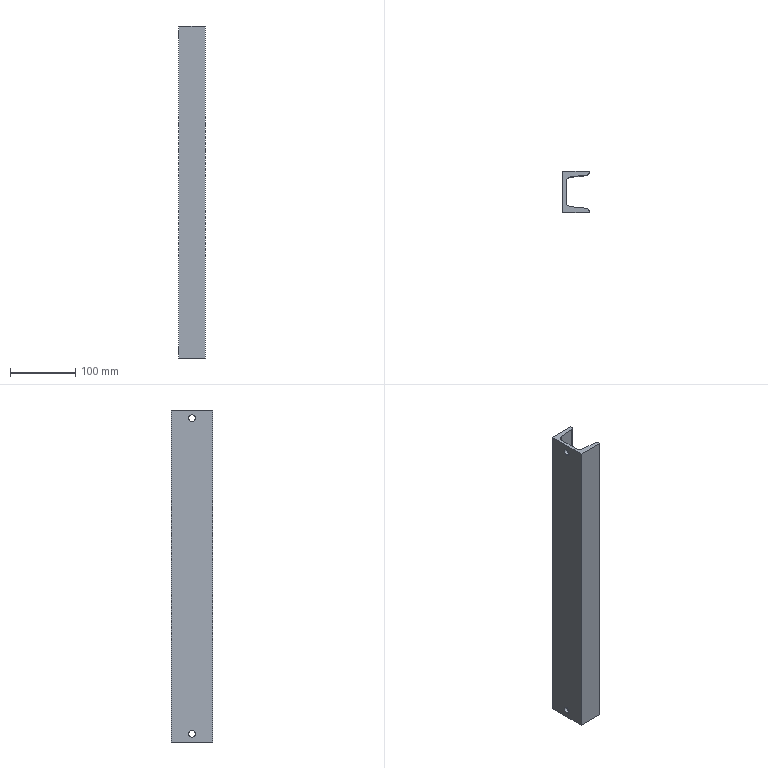Part | STEP file | 750038228 | 1 solid | 18 faces | box 40 x 63 x 510 mm | volume 429975 mm3 | plane 10 | cylinder 8 | commonest cylinder face diameters 10 x4 7.6 x2 15 x2
STEP:
#1=CARTESIAN_POINT('',(4.8,31.5,237.5));
#2=VERTEX_POINT('',#1);
#3=CARTESIAN_POINT('',(4.8,31.5,247.5));
#4=VERTEX_POINT('',#3);
#5=CARTESIAN_POINT('',(4.8,31.5,242.5));
#6=DIRECTION('',(-1.,0.,0.));
#7=DIRECTION('',(0.,0.,1.));
#8=AXIS2_PLACEMENT_3D('',#5,#6,#7);
#9=CIRCLE('',#8,5.);
#10=EDGE_CURVE('',#2,#4,#9,.T.);
#11=ORIENTED_EDGE('',*,*,#10,.F.);
#12=CARTESIAN_POINT('',(0.,31.5,237.5));
#13=VERTEX_POINT('',#12);
#14=CARTESIAN_POINT('',(55000.,31.5,237.5));
#15=DIRECTION('',(-1.,0.,0.));
#16=VECTOR('',#15,1000.);
#17=LINE('',#14,#16);
#18=EDGE_CURVE('',#2,#13,#17,.T.);
#19=ORIENTED_EDGE('',*,*,#18,.T.);
#20=CARTESIAN_POINT('',(0.,31.5,247.5));
#21=VERTEX_POINT('',#20);
#22=CARTESIAN_POINT('',(0.,31.5,242.5));
#23=DIRECTION('',(-1.,0.,0.));
#24=DIRECTION('',(0.,0.,1.));
#25=AXIS2_PLACEMENT_3D('',#22,#23,#24);
#26=CIRCLE('',#25,5.);
#27=EDGE_CURVE('',#13,#21,#26,.T.);
#28=ORIENTED_EDGE('',*,*,#27,.T.);
#29=CARTESIAN_POINT('',(55000.,31.5,247.5));
#30=DIRECTION('',(-1.,0.,0.));
#31=VECTOR('',#30,1000.);
#32=LINE('',#29,#31);
#33=EDGE_CURVE('',#4,#21,#32,.T.);
#34=ORIENTED_EDGE('',*,*,#33,.F.);
#35=EDGE_LOOP('',(#11,#19,#28,#34));
#36=FACE_OUTER_BOUND('',#35,.T.);
#37=CARTESIAN_POINT('',(55000.,31.5,242.5));
#38=DIRECTION('',(-1.,0.,0.));
#39=DIRECTION('',(0.,0.,1.));
#40=AXIS2_PLACEMENT_3D('',#37,#38,#39);
#41=CYLINDRICAL_SURFACE('',#40,5.);
#42=ADVANCED_FACE('',(#36),#41,.F.);
#43=CARTESIAN_POINT('',(4.8,31.5,-247.5));
#44=VERTEX_POINT('',#43);
#45=CARTESIAN_POINT('',(4.8,31.5,-237.5));
#46=VERTEX_POINT('',#45);
#47=CARTESIAN_POINT('',(4.8,31.5,-242.5));
#48=DIRECTION('',(-1.,0.,0.));
#49=DIRECTION('',(0.,0.,1.));
#50=AXIS2_PLACEMENT_3D('',#47,#48,#49);
#51=CIRCLE('',#50,5.);
#52=EDGE_CURVE('',#44,#46,#51,.T.);
#53=ORIENTED_EDGE('',*,*,#52,.F.);
#54=CARTESIAN_POINT('',(0.,31.5,-247.5));
#55=VERTEX_POINT('',#54);
#56=CARTESIAN_POINT('',(55000.,31.5,-247.5));
#57=DIRECTION('',(-1.,0.,0.));
#58=VECTOR('',#57,1000.);
#59=LINE('',#56,#58);
#60=EDGE_CURVE('',#44,#55,#59,.T.);
#61=ORIENTED_EDGE('',*,*,#60,.T.);
#62=CARTESIAN_POINT('',(0.,31.5,-237.5));
#63=VERTEX_POINT('',#62);
#64=CARTESIAN_POINT('',(0.,31.5,-242.5));
#65=DIRECTION('',(-1.,0.,0.));
#66=DIRECTION('',(0.,0.,1.));
#67=AXIS2_PLACEMENT_3D('',#64,#65,#66);
#68=CIRCLE('',#67,5.);
#69=EDGE_CURVE('',#55,#63,#68,.T.);
#70=ORIENTED_EDGE('',*,*,#69,.T.);
#71=CARTESIAN_POINT('',(55000.,31.5,-237.5));
#72=DIRECTION('',(-1.,0.,0.));
#73=VECTOR('',#72,1000.);
#74=LINE('',#71,#73);
#75=EDGE_CURVE('',#46,#63,#74,.T.);
#76=ORIENTED_EDGE('',*,*,#75,.F.);
#77=EDGE_LOOP('',(#53,#61,#70,#76));
#78=FACE_OUTER_BOUND('',#77,.T.);
#79=CARTESIAN_POINT('',(55000.,31.5,-242.5));
#80=DIRECTION('',(-1.,0.,0.));
#81=DIRECTION('',(0.,0.,1.));
#82=AXIS2_PLACEMENT_3D('',#79,#80,#81);
#83=CYLINDRICAL_SURFACE('',#82,5.);
#84=ADVANCED_FACE('',(#78),#83,.F.);
#85=CARTESIAN_POINT('',(0.,31.5,242.5));
#86=DIRECTION('',(-1.,0.,0.));
#87=DIRECTION('',(0.,0.,1.));
#88=AXIS2_PLACEMENT_3D('',#85,#86,#87);
#89=CIRCLE('',#88,5.);
#90=EDGE_CURVE('',#21,#13,#89,.T.);
#91=ORIENTED_EDGE('',*,*,#90,.F.);
#92=ORIENTED_EDGE('',*,*,#27,.F.);
#93=EDGE_LOOP('',(#91,#92));
#94=FACE_BOUND('',#93,.T.);
#95=CARTESIAN_POINT('',(0.,31.5,-242.5));
#96=DIRECTION('',(-1.,0.,0.));
#97=DIRECTION('',(0.,0.,1.));
#98=AXIS2_PLACEMENT_3D('',#95,#96,#97);
#99=CIRCLE('',#98,5.);
#100=EDGE_CURVE('',#63,#55,#99,.T.);
#101=ORIENTED_EDGE('',*,*,#100,.F.);
#102=ORIENTED_EDGE('',*,*,#69,.F.);
#103=EDGE_LOOP('',(#101,#102));
#104=FACE_BOUND('',#103,.T.);
#105=CARTESIAN_POINT('',(0.,0.,255.));
#106=VERTEX_POINT('',#105);
#107=CARTESIAN_POINT('',(0.,0.,-255.));
#108=VERTEX_POINT('',#107);
#109=CARTESIAN_POINT('',(0.,0.,255.));
#110=DIRECTION('',(0.,0.,-1.));
#111=VECTOR('',#110,1000.);
#112=LINE('',#109,#111);
#113=EDGE_CURVE('',#106,#108,#112,.T.);
#114=ORIENTED_EDGE('',*,*,#113,.F.);
#115=CARTESIAN_POINT('',(0.,63.,255.));
#116=VERTEX_POINT('',#115);
#117=CARTESIAN_POINT('',(0.,63.,255.));
#118=DIRECTION('',(0.,-1.,0.));
#119=VECTOR('',#118,1000.);
#120=LINE('',#117,#119);
#121=EDGE_CURVE('',#116,#106,#120,.T.);
#122=ORIENTED_EDGE('',*,*,#121,.F.);
#123=CARTESIAN_POINT('',(0.,63.,-255.));
#124=VERTEX_POINT('',#123);
#125=CARTESIAN_POINT('',(0.,63.,255.));
#126=DIRECTION('',(0.,0.,1.));
#127=VECTOR('',#126,1000.);
#128=LINE('',#125,#127);
#129=EDGE_CURVE('',#124,#116,#128,.T.);
#130=ORIENTED_EDGE('',*,*,#129,.F.);
#131=CARTESIAN_POINT('',(0.,63.,-255.));
#132=DIRECTION('',(0.,1.,0.));
#133=VECTOR('',#132,1000.);
#134=LINE('',#131,#133);
#135=EDGE_CURVE('',#108,#124,#134,.T.);
#136=ORIENTED_EDGE('',*,*,#135,.F.);
#137=EDGE_LOOP('',(#114,#122,#130,#136));
#138=FACE_OUTER_BOUND('',#137,.T.);
#139=CARTESIAN_POINT('',(0.,63.,255.));
#140=DIRECTION('',(1.,0.,0.));
#141=DIRECTION('',(0.,0.,-1.));
#142=AXIS2_PLACEMENT_3D('',#139,#140,#141);
#143=PLANE('',#142);
#144=ADVANCED_FACE('',(#94,#104,#138),#143,.F.);
#145=ORIENTED_EDGE('',*,*,#18,.F.);
#146=CARTESIAN_POINT('',(4.8,31.5,242.5));
#147=DIRECTION('',(-1.,0.,0.));
#148=DIRECTION('',(0.,0.,1.));
#149=AXIS2_PLACEMENT_3D('',#146,#147,#148);
#150=CIRCLE('',#149,5.);
#151=EDGE_CURVE('',#4,#2,#150,.T.);
#152=ORIENTED_EDGE('',*,*,#151,.F.);
#153=ORIENTED_EDGE('',*,*,#33,.T.);
#154=ORIENTED_EDGE('',*,*,#90,.T.);
#155=EDGE_LOOP('',(#145,#152,#153,#154));
#156=FACE_OUTER_BOUND('',#155,.T.);
#157=CARTESIAN_POINT('',(55000.,31.5,242.5));
#158=DIRECTION('',(-1.,0.,0.));
#159=DIRECTION('',(0.,0.,1.));
#160=AXIS2_PLACEMENT_3D('',#157,#158,#159);
#161=CYLINDRICAL_SURFACE('',#160,5.);
#162=ADVANCED_FACE('',(#156),#161,.F.);
#163=ORIENTED_EDGE('',*,*,#60,.F.);
#164=CARTESIAN_POINT('',(4.8,31.5,-242.5));
#165=DIRECTION('',(-1.,0.,0.));
#166=DIRECTION('',(0.,0.,1.));
#167=AXIS2_PLACEMENT_3D('',#164,#165,#166);
#168=CIRCLE('',#167,5.);
#169=EDGE_CURVE('',#46,#44,#168,.T.);
#170=ORIENTED_EDGE('',*,*,#169,.F.);
#171=ORIENTED_EDGE('',*,*,#75,.T.);
#172=ORIENTED_EDGE('',*,*,#100,.T.);
#173=EDGE_LOOP('',(#163,#170,#171,#172));
#174=FACE_OUTER_BOUND('',#173,.T.);
#175=CARTESIAN_POINT('',(55000.,31.5,-242.5));
#176=DIRECTION('',(-1.,0.,0.));
#177=DIRECTION('',(0.,0.,1.));
#178=AXIS2_PLACEMENT_3D('',#175,#176,#177);
#179=CYLINDRICAL_SURFACE('',#178,5.);
#180=ADVANCED_FACE('',(#174),#179,.F.);
#181=CARTESIAN_POINT('',(40.,63.,-255.));
#182=VERTEX_POINT('',#181);
#183=CARTESIAN_POINT('',(36.2,63.,-255.));
#184=DIRECTION('',(-1.,0.,0.));
#185=VECTOR('',#184,1000.);
#186=LINE('',#183,#185);
#187=EDGE_CURVE('',#182,#124,#186,.T.);
#188=ORIENTED_EDGE('',*,*,#187,.F.);
#189=CARTESIAN_POINT('',(40.,60.699,-255.));
#190=VERTEX_POINT('',#189);
#191=CARTESIAN_POINT('',(40.,2.301,-255.));
#192=DIRECTION('',(0.,1.,0.));
#193=VECTOR('',#192,1000.);
#194=LINE('',#191,#193);
#195=EDGE_CURVE('',#190,#182,#194,.T.);
#196=ORIENTED_EDGE('',*,*,#195,.F.);
#197=CARTESIAN_POINT('',(36.578,56.918,-255.));
#198=VERTEX_POINT('',#197);
#199=CARTESIAN_POINT('',(36.2,60.699,-255.));
#200=DIRECTION('',(0.,0.,1.));
#201=DIRECTION('',(-1.,0.,0.));
#202=AXIS2_PLACEMENT_3D('',#199,#200,#201);
#203=CIRCLE('',#202,3.8);
#204=EDGE_CURVE('',#198,#190,#203,.T.);
#205=ORIENTED_EDGE('',*,*,#204,.F.);
#206=CARTESIAN_POINT('',(11.554,54.415,-255.));
#207=VERTEX_POINT('',#206);
#208=CARTESIAN_POINT('',(11.554,54.415,-255.));
#209=DIRECTION('',(0.995,0.0995,0.));
#210=VECTOR('',#209,1000.);
#211=LINE('',#208,#210);
#212=EDGE_CURVE('',#207,#198,#211,.T.);
#213=ORIENTED_EDGE('',*,*,#212,.F.);
#214=CARTESIAN_POINT('',(4.8,46.953,-255.));
#215=VERTEX_POINT('',#214);
#216=CARTESIAN_POINT('',(12.3,46.953,-255.));
#217=DIRECTION('',(0.,0.,-1.));
#218=DIRECTION('',(-1.,0.,0.));
#219=AXIS2_PLACEMENT_3D('',#216,#217,#218);
#220=CIRCLE('',#219,7.5);
#221=EDGE_CURVE('',#215,#207,#220,.T.);
#222=ORIENTED_EDGE('',*,*,#221,.F.);
#223=CARTESIAN_POINT('',(4.8,16.047,-255.));
#224=VERTEX_POINT('',#223);
#225=CARTESIAN_POINT('',(4.8,2.301,-255.));
#226=DIRECTION('',(0.,1.,0.));
#227=VECTOR('',#226,1000.);
#228=LINE('',#225,#227);
#229=EDGE_CURVE('',#224,#215,#228,.T.);
#230=ORIENTED_EDGE('',*,*,#229,.F.);
#231=CARTESIAN_POINT('',(11.554,8.585,-255.));
#232=VERTEX_POINT('',#231);
#233=CARTESIAN_POINT('',(12.3,16.047,-255.));
#234=DIRECTION('',(0.,0.,-1.));
#235=DIRECTION('',(-1.,0.,0.));
#236=AXIS2_PLACEMENT_3D('',#233,#234,#235);
#237=CIRCLE('',#236,7.5);
#238=EDGE_CURVE('',#232,#224,#237,.T.);
#239=ORIENTED_EDGE('',*,*,#238,.F.);
#240=CARTESIAN_POINT('',(36.578,6.082,-255.));
#241=VERTEX_POINT('',#240);
#242=CARTESIAN_POINT('',(36.578,6.082,-255.));
#243=DIRECTION('',(-0.995,0.0995,0.));
#244=VECTOR('',#243,1000.);
#245=LINE('',#242,#244);
#246=EDGE_CURVE('',#241,#232,#245,.T.);
#247=ORIENTED_EDGE('',*,*,#246,.F.);
#248=CARTESIAN_POINT('',(40.,2.301,-255.));
#249=VERTEX_POINT('',#248);
#250=CARTESIAN_POINT('',(36.2,2.301,-255.));
#251=DIRECTION('',(0.,0.,1.));
#252=DIRECTION('',(-1.,0.,0.));
#253=AXIS2_PLACEMENT_3D('',#250,#251,#252);
#254=CIRCLE('',#253,3.8);
#255=EDGE_CURVE('',#249,#241,#254,.T.);
#256=ORIENTED_EDGE('',*,*,#255,.F.);
#257=CARTESIAN_POINT('',(40.,0.,-255.));
#258=VERTEX_POINT('',#257);
#259=CARTESIAN_POINT('',(40.,2.301,-255.));
#260=DIRECTION('',(0.,1.,0.));
#261=VECTOR('',#260,1000.);
#262=LINE('',#259,#261);
#263=EDGE_CURVE('',#258,#249,#262,.T.);
#264=ORIENTED_EDGE('',*,*,#263,.F.);
#265=CARTESIAN_POINT('',(36.2,0.,-255.));
#266=DIRECTION('',(1.,0.,0.));
#267=VECTOR('',#266,1000.);
#268=LINE('',#265,#267);
#269=EDGE_CURVE('',#108,#258,#268,.T.);
#270=ORIENTED_EDGE('',*,*,#269,.F.);
#271=ORIENTED_EDGE('',*,*,#135,.T.);
#272=EDGE_LOOP('',(#188,#196,#205,#213,#222,#230,#239,#247,#256,#264,#270,#271));
#273=FACE_OUTER_BOUND('',#272,.T.);
#274=CARTESIAN_POINT('',(36.2,2.301,-255.));
#275=DIRECTION('',(0.,0.,1.));
#276=DIRECTION('',(1.,0.,0.));
#277=AXIS2_PLACEMENT_3D('',#274,#275,#276);
#278=PLANE('',#277);
#279=ADVANCED_FACE('',(#273),#278,.F.);
#280=CARTESIAN_POINT('',(40.,0.,255.));
#281=VERTEX_POINT('',#280);
#282=CARTESIAN_POINT('',(40.,0.,255.));
#283=DIRECTION('',(0.,0.,-1.));
#284=VECTOR('',#283,1000.);
#285=LINE('',#282,#284);
#286=EDGE_CURVE('',#281,#258,#285,.T.);
#287=ORIENTED_EDGE('',*,*,#286,.F.);
#288=CARTESIAN_POINT('',(0.,0.,255.));
#289=DIRECTION('',(1.,0.,0.));
#290=VECTOR('',#289,1000.);
#291=LINE('',#288,#290);
#292=EDGE_CURVE('',#106,#281,#291,.T.);
#293=ORIENTED_EDGE('',*,*,#292,.F.);
#294=ORIENTED_EDGE('',*,*,#113,.T.);
#295=ORIENTED_EDGE('',*,*,#269,.T.);
#296=EDGE_LOOP('',(#287,#293,#294,#295));
#297=FACE_OUTER_BOUND('',#296,.T.);
#298=CARTESIAN_POINT('',(0.,0.,255.));
#299=DIRECTION('',(0.,1.,0.));
#300=DIRECTION('',(0.,0.,1.));
#301=AXIS2_PLACEMENT_3D('',#298,#299,#300);
#302=PLANE('',#301);
#303=ADVANCED_FACE('',(#297),#302,.F.);
#304=CARTESIAN_POINT('',(40.,60.699,255.));
#305=VERTEX_POINT('',#304);
#306=CARTESIAN_POINT('',(40.,63.,255.));
#307=VERTEX_POINT('',#306);
#308=CARTESIAN_POINT('',(40.,2.301,255.));
#309=DIRECTION('',(0.,1.,0.));
#310=VECTOR('',#309,1000.);
#311=LINE('',#308,#310);
#312=EDGE_CURVE('',#305,#307,#311,.T.);
#313=ORIENTED_EDGE('',*,*,#312,.T.);
#314=CARTESIAN_POINT('',(36.2,63.,255.));
#315=DIRECTION('',(-1.,0.,0.));
#316=VECTOR('',#315,1000.);
#317=LINE('',#314,#316);
#318=EDGE_CURVE('',#307,#116,#317,.T.);
#319=ORIENTED_EDGE('',*,*,#318,.T.);
#320=ORIENTED_EDGE('',*,*,#121,.T.);
#321=ORIENTED_EDGE('',*,*,#292,.T.);
#322=CARTESIAN_POINT('',(40.,2.301,255.));
#323=VERTEX_POINT('',#322);
#324=CARTESIAN_POINT('',(40.,2.301,255.));
#325=DIRECTION('',(0.,1.,0.));
#326=VECTOR('',#325,1000.);
#327=LINE('',#324,#326);
#328=EDGE_CURVE('',#281,#323,#327,.T.);
#329=ORIENTED_EDGE('',*,*,#328,.T.);
#330=CARTESIAN_POINT('',(36.578,6.082,255.));
#331=VERTEX_POINT('',#330);
#332=CARTESIAN_POINT('',(36.2,2.301,255.));
#333=DIRECTION('',(0.,0.,1.));
#334=DIRECTION('',(-1.,0.,0.));
#335=AXIS2_PLACEMENT_3D('',#332,#333,#334);
#336=CIRCLE('',#335,3.8);
#337=EDGE_CURVE('',#323,#331,#336,.T.);
#338=ORIENTED_EDGE('',*,*,#337,.T.);
#339=CARTESIAN_POINT('',(11.554,8.585,255.));
#340=VERTEX_POINT('',#339);
#341=CARTESIAN_POINT('',(36.578,6.082,255.));
#342=DIRECTION('',(-0.995,0.0995,0.));
#343=VECTOR('',#342,1000.);
#344=LINE('',#341,#343);
#345=EDGE_CURVE('',#331,#340,#344,.T.);
#346=ORIENTED_EDGE('',*,*,#345,.T.);
#347=CARTESIAN_POINT('',(4.8,16.047,255.));
#348=VERTEX_POINT('',#347);
#349=CARTESIAN_POINT('',(12.3,16.047,255.));
#350=DIRECTION('',(0.,0.,-1.));
#351=DIRECTION('',(-1.,0.,0.));
#352=AXIS2_PLACEMENT_3D('',#349,#350,#351);
#353=CIRCLE('',#352,7.5);
#354=EDGE_CURVE('',#340,#348,#353,.T.);
#355=ORIENTED_EDGE('',*,*,#354,.T.);
#356=CARTESIAN_POINT('',(4.8,46.953,255.));
#357=VERTEX_POINT('',#356);
#358=CARTESIAN_POINT('',(4.8,2.301,255.));
#359=DIRECTION('',(0.,1.,0.));
#360=VECTOR('',#359,1000.);
#361=LINE('',#358,#360);
#362=EDGE_CURVE('',#348,#357,#361,.T.);
#363=ORIENTED_EDGE('',*,*,#362,.T.);
#364=CARTESIAN_POINT('',(11.554,54.415,255.));
#365=VERTEX_POINT('',#364);
#366=CARTESIAN_POINT('',(12.3,46.953,255.));
#367=DIRECTION('',(0.,0.,-1.));
#368=DIRECTION('',(-1.,0.,0.));
#369=AXIS2_PLACEMENT_3D('',#366,#367,#368);
#370=CIRCLE('',#369,7.5);
#371=EDGE_CURVE('',#357,#365,#370,.T.);
#372=ORIENTED_EDGE('',*,*,#371,.T.);
#373=CARTESIAN_POINT('',(36.578,56.918,255.));
#374=VERTEX_POINT('',#373);
#375=CARTESIAN_POINT('',(11.554,54.415,255.));
#376=DIRECTION('',(0.995,0.0995,0.));
#377=VECTOR('',#376,1000.);
#378=LINE('',#375,#377);
#379=EDGE_CURVE('',#365,#374,#378,.T.);
#380=ORIENTED_EDGE('',*,*,#379,.T.);
#381=CARTESIAN_POINT('',(36.2,60.699,255.));
#382=DIRECTION('',(0.,0.,1.));
#383=DIRECTION('',(-1.,0.,0.));
#384=AXIS2_PLACEMENT_3D('',#381,#382,#383);
#385=CIRCLE('',#384,3.8);
#386=EDGE_CURVE('',#374,#305,#385,.T.);
#387=ORIENTED_EDGE('',*,*,#386,.T.);
#388=EDGE_LOOP('',(#313,#319,#320,#321,#329,#338,#346,#355,#363,#372,#380,#387));
#389=FACE_OUTER_BOUND('',#388,.T.);
#390=CARTESIAN_POINT('',(36.2,2.301,255.));
#391=DIRECTION('',(0.,0.,1.));
#392=DIRECTION('',(1.,0.,0.));
#393=AXIS2_PLACEMENT_3D('',#390,#391,#392);
#394=PLANE('',#393);
#395=ADVANCED_FACE('',(#389),#394,.T.);
#396=ORIENTED_EDGE('',*,*,#129,.T.);
#397=ORIENTED_EDGE('',*,*,#318,.F.);
#398=CARTESIAN_POINT('',(40.,63.,255.));
#399=DIRECTION('',(0.,0.,1.));
#400=VECTOR('',#399,1000.);
#401=LINE('',#398,#400);
#402=EDGE_CURVE('',#182,#307,#401,.T.);
#403=ORIENTED_EDGE('',*,*,#402,.F.);
#404=ORIENTED_EDGE('',*,*,#187,.T.);
#405=EDGE_LOOP('',(#396,#397,#403,#404));
#406=FACE_OUTER_BOUND('',#405,.T.);
#407=CARTESIAN_POINT('',(40.,63.,255.));
#408=DIRECTION('',(0.,-1.,0.));
#409=DIRECTION('',(0.,0.,-1.));
#410=AXIS2_PLACEMENT_3D('',#407,#408,#409);
#411=PLANE('',#410);
#412=ADVANCED_FACE('',(#406),#411,.F.);
#413=ORIENTED_EDGE('',*,*,#151,.T.);
#414=ORIENTED_EDGE('',*,*,#10,.T.);
#415=EDGE_LOOP('',(#413,#414));
#416=FACE_BOUND('',#415,.T.);
#417=CARTESIAN_POINT('',(4.8,46.953,255.));
#418=DIRECTION('',(0.,0.,-1.));
#419=VECTOR('',#418,1000.);
#420=LINE('',#417,#419);
#421=EDGE_CURVE('',#357,#215,#420,.T.);
#422=ORIENTED_EDGE('',*,*,#421,.F.);
#423=ORIENTED_EDGE('',*,*,#362,.F.);
#424=CARTESIAN_POINT('',(4.8,16.047,255.));
#425=DIRECTION('',(0.,0.,1.));
#426=VECTOR('',#425,1000.);
#427=LINE('',#424,#426);
#428=EDGE_CURVE('',#224,#348,#427,.T.);
#429=ORIENTED_EDGE('',*,*,#428,.F.);
#430=ORIENTED_EDGE('',*,*,#229,.T.);
#431=EDGE_LOOP('',(#422,#423,#429,#430));
#432=FACE_OUTER_BOUND('',#431,.T.);
#433=ORIENTED_EDGE('',*,*,#169,.T.);
#434=ORIENTED_EDGE('',*,*,#52,.T.);
#435=EDGE_LOOP('',(#433,#434));
#436=FACE_BOUND('',#435,.T.);
#437=CARTESIAN_POINT('',(4.8,16.047,255.));
#438=DIRECTION('',(-1.,0.,0.));
#439=DIRECTION('',(0.,-1.,0.));
#440=AXIS2_PLACEMENT_3D('',#437,#438,#439);
#441=PLANE('',#440);
#442=ADVANCED_FACE('',(#416,#432,#436),#441,.F.);
#443=ORIENTED_EDGE('',*,*,#402,.T.);
#444=ORIENTED_EDGE('',*,*,#312,.F.);
#445=CARTESIAN_POINT('',(40.,60.699,255.));
#446=DIRECTION('',(0.,0.,1.));
#447=VECTOR('',#446,1000.);
#448=LINE('',#445,#447);
#449=EDGE_CURVE('',#190,#305,#448,.T.);
#450=ORIENTED_EDGE('',*,*,#449,.F.);
#451=ORIENTED_EDGE('',*,*,#195,.T.);
#452=EDGE_LOOP('',(#443,#444,#450,#451));
#453=FACE_OUTER_BOUND('',#452,.T.);
#454=CARTESIAN_POINT('',(40.,60.699,255.));
#455=DIRECTION('',(-1.,0.,0.));
#456=DIRECTION('',(0.,-1.,0.));
#457=AXIS2_PLACEMENT_3D('',#454,#455,#456);
#458=PLANE('',#457);
#459=ADVANCED_FACE('',(#453),#458,.F.);
#460=ORIENTED_EDGE('',*,*,#386,.F.);
#461=CARTESIAN_POINT('',(36.578,56.918,255.));
#462=DIRECTION('',(0.,0.,-1.));
#463=VECTOR('',#462,1000.);
#464=LINE('',#461,#463);
#465=EDGE_CURVE('',#374,#198,#464,.T.);
#466=ORIENTED_EDGE('',*,*,#465,.T.);
#467=ORIENTED_EDGE('',*,*,#204,.T.);
#468=ORIENTED_EDGE('',*,*,#449,.T.);
#469=EDGE_LOOP('',(#460,#466,#467,#468));
#470=FACE_OUTER_BOUND('',#469,.T.);
#471=CARTESIAN_POINT('',(36.2,60.699,255.));
#472=DIRECTION('',(0.,0.,-1.));
#473=DIRECTION('',(-1.,0.,0.));
#474=AXIS2_PLACEMENT_3D('',#471,#472,#473);
#475=CYLINDRICAL_SURFACE('',#474,3.8);
#476=ADVANCED_FACE('',(#470),#475,.T.);
#477=ORIENTED_EDGE('',*,*,#465,.F.);
#478=ORIENTED_EDGE('',*,*,#379,.F.);
#479=CARTESIAN_POINT('',(11.554,54.415,255.));
#480=DIRECTION('',(0.,0.,1.));
#481=VECTOR('',#480,1000.);
#482=LINE('',#479,#481);
#483=EDGE_CURVE('',#207,#365,#482,.T.);
#484=ORIENTED_EDGE('',*,*,#483,.F.);
#485=ORIENTED_EDGE('',*,*,#212,.T.);
#486=EDGE_LOOP('',(#477,#478,#484,#485));
#487=FACE_OUTER_BOUND('',#486,.T.);
#488=CARTESIAN_POINT('',(11.554,54.415,255.));
#489=DIRECTION('',(-0.0995,0.995,0.));
#490=DIRECTION('',(-0.995,-0.0995,0.));
#491=AXIS2_PLACEMENT_3D('',#488,#489,#490);
#492=PLANE('',#491);
#493=ADVANCED_FACE('',(#487),#492,.F.);
#494=ORIENTED_EDGE('',*,*,#483,.T.);
#495=ORIENTED_EDGE('',*,*,#371,.F.);
#496=ORIENTED_EDGE('',*,*,#421,.T.);
#497=ORIENTED_EDGE('',*,*,#221,.T.);
#498=EDGE_LOOP('',(#494,#495,#496,#497));
#499=FACE_OUTER_BOUND('',#498,.T.);
#500=CARTESIAN_POINT('',(12.3,46.953,255.));
#501=DIRECTION('',(0.,0.,-1.));
#502=DIRECTION('',(-1.,0.,0.));
#503=AXIS2_PLACEMENT_3D('',#500,#501,#502);
#504=CYLINDRICAL_SURFACE('',#503,7.5);
#505=ADVANCED_FACE('',(#499),#504,.F.);
#506=ORIENTED_EDGE('',*,*,#428,.T.);
#507=ORIENTED_EDGE('',*,*,#354,.F.);
#508=CARTESIAN_POINT('',(11.554,8.585,255.));
#509=DIRECTION('',(0.,0.,1.));
#510=VECTOR('',#509,1000.);
#511=LINE('',#508,#510);
#512=EDGE_CURVE('',#232,#340,#511,.T.);
#513=ORIENTED_EDGE('',*,*,#512,.F.);
#514=ORIENTED_EDGE('',*,*,#238,.T.);
#515=EDGE_LOOP('',(#506,#507,#513,#514));
#516=FACE_OUTER_BOUND('',#515,.T.);
#517=CARTESIAN_POINT('',(12.3,16.047,255.));
#518=DIRECTION('',(0.,0.,-1.));
#519=DIRECTION('',(-1.,0.,0.));
#520=AXIS2_PLACEMENT_3D('',#517,#518,#519);
#521=CYLINDRICAL_SURFACE('',#520,7.5);
#522=ADVANCED_FACE('',(#516),#521,.F.);
#523=ORIENTED_EDGE('',*,*,#512,.T.);
#524=ORIENTED_EDGE('',*,*,#345,.F.);
#525=CARTESIAN_POINT('',(36.578,6.082,255.));
#526=DIRECTION('',(0.,0.,1.));
#527=VECTOR('',#526,1000.);
#528=LINE('',#525,#527);
#529=EDGE_CURVE('',#241,#331,#528,.T.);
#530=ORIENTED_EDGE('',*,*,#529,.F.);
#531=ORIENTED_EDGE('',*,*,#246,.T.);
#532=EDGE_LOOP('',(#523,#524,#530,#531));
#533=FACE_OUTER_BOUND('',#532,.T.);
#534=CARTESIAN_POINT('',(36.578,6.082,255.));
#535=DIRECTION('',(-0.0995,-0.995,0.));
#536=DIRECTION('',(0.995,-0.0995,0.));
#537=AXIS2_PLACEMENT_3D('',#534,#535,#536);
#538=PLANE('',#537);
#539=ADVANCED_FACE('',(#533),#538,.F.);
#540=ORIENTED_EDGE('',*,*,#337,.F.);
#541=CARTESIAN_POINT('',(40.,2.301,255.));
#542=DIRECTION('',(0.,0.,-1.));
#543=VECTOR('',#542,1000.);
#544=LINE('',#541,#543);
#545=EDGE_CURVE('',#323,#249,#544,.T.);
#546=ORIENTED_EDGE('',*,*,#545,.T.);
#547=ORIENTED_EDGE('',*,*,#255,.T.);
#548=ORIENTED_EDGE('',*,*,#529,.T.);
#549=EDGE_LOOP('',(#540,#546,#547,#548));
#550=FACE_OUTER_BOUND('',#549,.T.);
#551=CARTESIAN_POINT('',(36.2,2.301,255.));
#552=DIRECTION('',(0.,0.,-1.));
#553=DIRECTION('',(-1.,0.,0.));
#554=AXIS2_PLACEMENT_3D('',#551,#552,#553);
#555=CYLINDRICAL_SURFACE('',#554,3.8);
#556=ADVANCED_FACE('',(#550),#555,.T.);
#557=ORIENTED_EDGE('',*,*,#545,.F.);
#558=ORIENTED_EDGE('',*,*,#328,.F.);
#559=ORIENTED_EDGE('',*,*,#286,.T.);
#560=ORIENTED_EDGE('',*,*,#263,.T.);
#561=EDGE_LOOP('',(#557,#558,#559,#560));
#562=FACE_OUTER_BOUND('',#561,.T.);
#563=CARTESIAN_POINT('',(40.,0.,255.));
#564=DIRECTION('',(-1.,0.,0.));
#565=DIRECTION('',(0.,0.,1.));
#566=AXIS2_PLACEMENT_3D('',#563,#564,#565);
#567=PLANE('',#566);
#568=ADVANCED_FACE('',(#562),#567,.F.);
#569=CLOSED_SHELL('',(#42,#84,#144,#162,#180,#279,#303,#395,#412,#442,#459,#476,#493,#505,#522,#539,#556,#568));
#570=MANIFOLD_SOLID_BREP('',#569);
#571=CARTESIAN_POINT('',(0.,0.,0.));
#572=DIRECTION('',(0.,0.,1.));
#573=DIRECTION('',(1.,0.,0.));
#574=AXIS2_PLACEMENT_3D('',#571,#572,#573);
#575=(LENGTH_UNIT()NAMED_UNIT(*)SI_UNIT(.MILLI.,.METRE.));
#576=UNCERTAINTY_MEASURE_WITH_UNIT(LENGTH_MEASURE(0.00001),#575,'','');
#577=(NAMED_UNIT(*)PLANE_ANGLE_UNIT()SI_UNIT($,.RADIAN.));
#578=(NAMED_UNIT(*)SI_UNIT($,.STERADIAN.)SOLID_ANGLE_UNIT());
#579=(GEOMETRIC_REPRESENTATION_CONTEXT(3)GLOBAL_UNCERTAINTY_ASSIGNED_CONTEXT((#576))GLOBAL_UNIT_ASSIGNED_CONTEXT((#575,#577,#578))REPRESENTATION_CONTEXT('',''));
#580=ADVANCED_BREP_SHAPE_REPRESENTATION('',(#570,#574),#579);